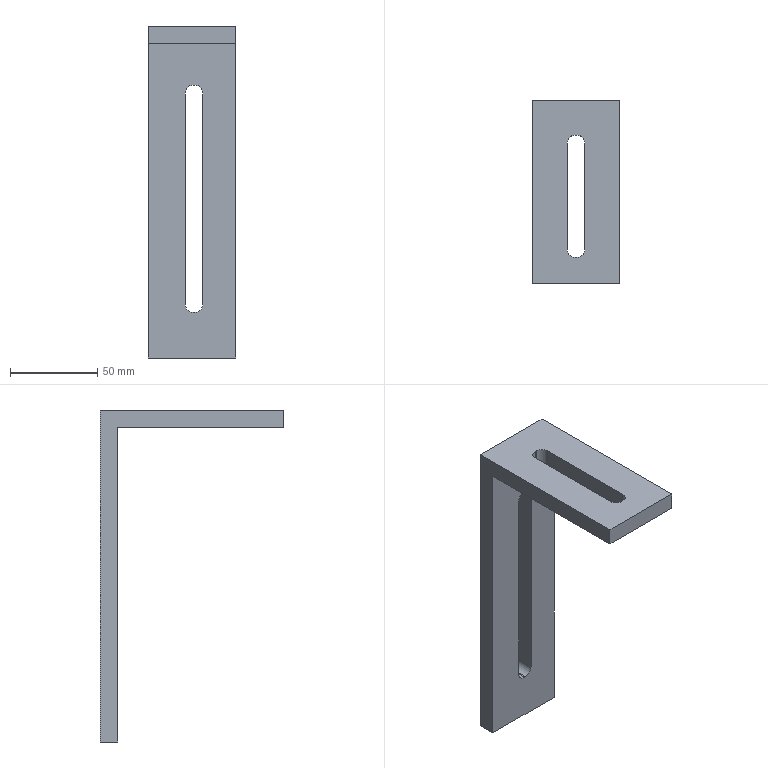Part | SolidWorks | features ICE 3, Extrusion 1 | 1 solid | 24 faces | box 50 x 105 x 190 mm | volume 122848 mm3 | plane 16 | cylinder 8 | commonest cylinder face diameters 9 x8
STEP:
#1=CARTESIAN_POINT('',(-25.,-50.,10.));
#2=VERTEX_POINT('',#1);
#3=CARTESIAN_POINT('',(-25.,-50.,0.));
#4=VERTEX_POINT('',#3);
#5=CARTESIAN_POINT('',(-25.,-50.,10.));
#6=DIRECTION('',(0.,0.,-1.));
#7=VECTOR('',#6,1000.);
#8=LINE('',#5,#7);
#9=EDGE_CURVE('',#2,#4,#8,.T.);
#10=ORIENTED_EDGE('',*,*,#9,.F.);
#11=CARTESIAN_POINT('',(-25.,55.,10.));
#12=VERTEX_POINT('',#11);
#13=CARTESIAN_POINT('',(-25.,-50.,10.));
#14=DIRECTION('',(0.,-1.,0.));
#15=VECTOR('',#14,1000.);
#16=LINE('',#13,#15);
#17=EDGE_CURVE('',#12,#2,#16,.T.);
#18=ORIENTED_EDGE('',*,*,#17,.F.);
#19=CARTESIAN_POINT('',(-25.,55.,-180.));
#20=VERTEX_POINT('',#19);
#21=CARTESIAN_POINT('',(-25.,55.,10.));
#22=DIRECTION('',(0.,0.,-1.));
#23=VECTOR('',#22,1000.);
#24=LINE('',#21,#23);
#25=EDGE_CURVE('',#12,#20,#24,.T.);
#26=ORIENTED_EDGE('',*,*,#25,.T.);
#27=CARTESIAN_POINT('',(-25.,45.,-180.));
#28=VERTEX_POINT('',#27);
#29=CARTESIAN_POINT('',(-25.,45.,-180.));
#30=DIRECTION('',(0.,1.,0.));
#31=VECTOR('',#30,1000.);
#32=LINE('',#29,#31);
#33=EDGE_CURVE('',#28,#20,#32,.T.);
#34=ORIENTED_EDGE('',*,*,#33,.F.);
#35=CARTESIAN_POINT('',(-25.,45.,0.));
#36=VERTEX_POINT('',#35);
#37=CARTESIAN_POINT('',(-25.,45.,10.));
#38=DIRECTION('',(0.,0.,-1.));
#39=VECTOR('',#38,1000.);
#40=LINE('',#37,#39);
#41=EDGE_CURVE('',#36,#28,#40,.T.);
#42=ORIENTED_EDGE('',*,*,#41,.F.);
#43=CARTESIAN_POINT('',(-25.,-50.,0.));
#44=DIRECTION('',(0.,-1.,0.));
#45=VECTOR('',#44,1000.);
#46=LINE('',#43,#45);
#47=EDGE_CURVE('',#36,#4,#46,.T.);
#48=ORIENTED_EDGE('',*,*,#47,.T.);
#49=EDGE_LOOP('',(#10,#18,#26,#34,#42,#48));
#50=FACE_OUTER_BOUND('',#49,.T.);
#51=CARTESIAN_POINT('',(-25.,-50.,10.));
#52=DIRECTION('',(1.,0.,0.));
#53=DIRECTION('',(0.,0.,-1.));
#54=AXIS2_PLACEMENT_3D('',#51,#52,#53);
#55=PLANE('',#54);
#56=ADVANCED_FACE('',(#50),#55,.F.);
#57=CARTESIAN_POINT('',(25.,-50.,0.));
#58=VERTEX_POINT('',#57);
#59=CARTESIAN_POINT('',(25.,-50.,0.));
#60=DIRECTION('',(1.,0.,0.));
#61=VECTOR('',#60,1000.);
#62=LINE('',#59,#61);
#63=EDGE_CURVE('',#4,#58,#62,.T.);
#64=ORIENTED_EDGE('',*,*,#63,.T.);
#65=CARTESIAN_POINT('',(25.,-50.,10.));
#66=VERTEX_POINT('',#65);
#67=CARTESIAN_POINT('',(25.,-50.,10.));
#68=DIRECTION('',(0.,0.,-1.));
#69=VECTOR('',#68,1000.);
#70=LINE('',#67,#69);
#71=EDGE_CURVE('',#66,#58,#70,.T.);
#72=ORIENTED_EDGE('',*,*,#71,.F.);
#73=CARTESIAN_POINT('',(25.,-50.,10.));
#74=DIRECTION('',(1.,0.,0.));
#75=VECTOR('',#74,1000.);
#76=LINE('',#73,#75);
#77=EDGE_CURVE('',#2,#66,#76,.T.);
#78=ORIENTED_EDGE('',*,*,#77,.F.);
#79=ORIENTED_EDGE('',*,*,#9,.T.);
#80=EDGE_LOOP('',(#64,#72,#78,#79));
#81=FACE_OUTER_BOUND('',#80,.T.);
#82=CARTESIAN_POINT('',(25.,-50.,10.));
#83=DIRECTION('',(0.,1.,0.));
#84=DIRECTION('',(0.,0.,1.));
#85=AXIS2_PLACEMENT_3D('',#82,#83,#84);
#86=PLANE('',#85);
#87=ADVANCED_FACE('',(#81),#86,.F.);
#88=CARTESIAN_POINT('',(25.,45.,0.));
#89=VERTEX_POINT('',#88);
#90=CARTESIAN_POINT('',(25.,-50.,0.));
#91=DIRECTION('',(0.,1.,0.));
#92=VECTOR('',#91,1000.);
#93=LINE('',#90,#92);
#94=EDGE_CURVE('',#58,#89,#93,.T.);
#95=ORIENTED_EDGE('',*,*,#94,.T.);
#96=CARTESIAN_POINT('',(25.,45.,-180.));
#97=VERTEX_POINT('',#96);
#98=CARTESIAN_POINT('',(25.,45.,10.));
#99=DIRECTION('',(0.,0.,-1.));
#100=VECTOR('',#99,1000.);
#101=LINE('',#98,#100);
#102=EDGE_CURVE('',#89,#97,#101,.T.);
#103=ORIENTED_EDGE('',*,*,#102,.T.);
#104=CARTESIAN_POINT('',(25.,55.,-180.));
#105=VERTEX_POINT('',#104);
#106=CARTESIAN_POINT('',(25.,45.,-180.));
#107=DIRECTION('',(0.,-1.,0.));
#108=VECTOR('',#107,1000.);
#109=LINE('',#106,#108);
#110=EDGE_CURVE('',#105,#97,#109,.T.);
#111=ORIENTED_EDGE('',*,*,#110,.F.);
#112=CARTESIAN_POINT('',(25.,55.,10.));
#113=VERTEX_POINT('',#112);
#114=CARTESIAN_POINT('',(25.,55.,10.));
#115=DIRECTION('',(0.,0.,-1.));
#116=VECTOR('',#115,1000.);
#117=LINE('',#114,#116);
#118=EDGE_CURVE('',#113,#105,#117,.T.);
#119=ORIENTED_EDGE('',*,*,#118,.F.);
#120=CARTESIAN_POINT('',(25.,-50.,10.));
#121=DIRECTION('',(0.,1.,0.));
#122=VECTOR('',#121,1000.);
#123=LINE('',#120,#122);
#124=EDGE_CURVE('',#66,#113,#123,.T.);
#125=ORIENTED_EDGE('',*,*,#124,.F.);
#126=ORIENTED_EDGE('',*,*,#71,.T.);
#127=EDGE_LOOP('',(#95,#103,#111,#119,#125,#126));
#128=FACE_OUTER_BOUND('',#127,.T.);
#129=CARTESIAN_POINT('',(25.,-50.,10.));
#130=DIRECTION('',(-1.,0.,0.));
#131=DIRECTION('',(0.,0.,1.));
#132=AXIS2_PLACEMENT_3D('',#129,#130,#131);
#133=PLANE('',#132);
#134=ADVANCED_FACE('',(#128),#133,.F.);
#135=ORIENTED_EDGE('',*,*,#124,.T.);
#136=CARTESIAN_POINT('',(-25.,55.,10.));
#137=DIRECTION('',(1.,0.,0.));
#138=VECTOR('',#137,1000.);
#139=LINE('',#136,#138);
#140=EDGE_CURVE('',#12,#113,#139,.T.);
#141=ORIENTED_EDGE('',*,*,#140,.F.);
#142=ORIENTED_EDGE('',*,*,#17,.T.);
#143=ORIENTED_EDGE('',*,*,#77,.T.);
#144=EDGE_LOOP('',(#135,#141,#142,#143));
#145=FACE_OUTER_BOUND('',#144,.T.);
#146=CARTESIAN_POINT('',(-5.,-30.5,10.));
#147=VERTEX_POINT('',#146);
#148=CARTESIAN_POINT('',(-0.5,-35.,10.));
#149=VERTEX_POINT('',#148);
#150=CARTESIAN_POINT('',(-0.5,-30.5,10.));
#151=DIRECTION('',(0.,0.,1.));
#152=DIRECTION('',(-1.,0.,0.));
#153=AXIS2_PLACEMENT_3D('',#150,#151,#152);
#154=CIRCLE('',#153,4.5);
#155=EDGE_CURVE('',#147,#149,#154,.T.);
#156=ORIENTED_EDGE('',*,*,#155,.F.);
#157=CARTESIAN_POINT('',(-5.,30.5,10.));
#158=VERTEX_POINT('',#157);
#159=CARTESIAN_POINT('',(-5.,-30.5,10.));
#160=DIRECTION('',(0.,-1.,0.));
#161=VECTOR('',#160,1000.);
#162=LINE('',#159,#161);
#163=EDGE_CURVE('',#158,#147,#162,.T.);
#164=ORIENTED_EDGE('',*,*,#163,.F.);
#165=CARTESIAN_POINT('',(-0.5,35.,10.));
#166=VERTEX_POINT('',#165);
#167=CARTESIAN_POINT('',(-0.5,30.5,10.));
#168=DIRECTION('',(0.,0.,1.));
#169=DIRECTION('',(1.,0.,0.));
#170=AXIS2_PLACEMENT_3D('',#167,#168,#169);
#171=CIRCLE('',#170,4.5);
#172=EDGE_CURVE('',#166,#158,#171,.T.);
#173=ORIENTED_EDGE('',*,*,#172,.F.);
#174=CARTESIAN_POINT('',(0.5,35.,10.));
#175=VERTEX_POINT('',#174);
#176=CARTESIAN_POINT('',(0.5,35.,10.));
#177=DIRECTION('',(-1.,0.,0.));
#178=VECTOR('',#177,1000.);
#179=LINE('',#176,#178);
#180=EDGE_CURVE('',#175,#166,#179,.T.);
#181=ORIENTED_EDGE('',*,*,#180,.F.);
#182=CARTESIAN_POINT('',(5.,30.5,10.));
#183=VERTEX_POINT('',#182);
#184=CARTESIAN_POINT('',(0.5,30.5,10.));
#185=DIRECTION('',(0.,0.,1.));
#186=DIRECTION('',(1.,0.,0.));
#187=AXIS2_PLACEMENT_3D('',#184,#185,#186);
#188=CIRCLE('',#187,4.5);
#189=EDGE_CURVE('',#183,#175,#188,.T.);
#190=ORIENTED_EDGE('',*,*,#189,.F.);
#191=CARTESIAN_POINT('',(5.,-30.5,10.));
#192=VERTEX_POINT('',#191);
#193=CARTESIAN_POINT('',(5.,-30.5,10.));
#194=DIRECTION('',(0.,1.,0.));
#195=VECTOR('',#194,1000.);
#196=LINE('',#193,#195);
#197=EDGE_CURVE('',#192,#183,#196,.T.);
#198=ORIENTED_EDGE('',*,*,#197,.F.);
#199=CARTESIAN_POINT('',(0.5,-35.,10.));
#200=VERTEX_POINT('',#199);
#201=CARTESIAN_POINT('',(0.5,-30.5,10.));
#202=DIRECTION('',(0.,0.,1.));
#203=DIRECTION('',(1.,0.,0.));
#204=AXIS2_PLACEMENT_3D('',#201,#202,#203);
#205=CIRCLE('',#204,4.5);
#206=EDGE_CURVE('',#200,#192,#205,.T.);
#207=ORIENTED_EDGE('',*,*,#206,.F.);
#208=CARTESIAN_POINT('',(0.5,-35.,10.));
#209=DIRECTION('',(1.,0.,0.));
#210=VECTOR('',#209,1000.);
#211=LINE('',#208,#210);
#212=EDGE_CURVE('',#149,#200,#211,.T.);
#213=ORIENTED_EDGE('',*,*,#212,.F.);
#214=EDGE_LOOP('',(#156,#164,#173,#181,#190,#198,#207,#213));
#215=FACE_BOUND('',#214,.T.);
#216=CARTESIAN_POINT('',(-25.,50.,10.));
#217=DIRECTION('',(0.,0.,1.));
#218=DIRECTION('',(1.,0.,0.));
#219=AXIS2_PLACEMENT_3D('',#216,#217,#218);
#220=PLANE('',#219);
#221=ADVANCED_FACE('',(#145,#215),#220,.T.);
#222=CARTESIAN_POINT('',(-5.,30.5,0.));
#223=VERTEX_POINT('',#222);
#224=CARTESIAN_POINT('',(-5.,-30.5,0.));
#225=VERTEX_POINT('',#224);
#226=CARTESIAN_POINT('',(-5.,-30.5,0.));
#227=DIRECTION('',(0.,-1.,0.));
#228=VECTOR('',#227,1000.);
#229=LINE('',#226,#228);
#230=EDGE_CURVE('',#223,#225,#229,.T.);
#231=ORIENTED_EDGE('',*,*,#230,.T.);
#232=CARTESIAN_POINT('',(-0.5,-35.,0.));
#233=VERTEX_POINT('',#232);
#234=CARTESIAN_POINT('',(-0.5,-30.5,0.));
#235=DIRECTION('',(0.,0.,1.));
#236=DIRECTION('',(-1.,0.,0.));
#237=AXIS2_PLACEMENT_3D('',#234,#235,#236);
#238=CIRCLE('',#237,4.5);
#239=EDGE_CURVE('',#225,#233,#238,.T.);
#240=ORIENTED_EDGE('',*,*,#239,.T.);
#241=CARTESIAN_POINT('',(0.5,-35.,0.));
#242=VERTEX_POINT('',#241);
#243=CARTESIAN_POINT('',(0.5,-35.,0.));
#244=DIRECTION('',(1.,0.,0.));
#245=VECTOR('',#244,1000.);
#246=LINE('',#243,#245);
#247=EDGE_CURVE('',#233,#242,#246,.T.);
#248=ORIENTED_EDGE('',*,*,#247,.T.);
#249=CARTESIAN_POINT('',(5.,-30.5,0.));
#250=VERTEX_POINT('',#249);
#251=CARTESIAN_POINT('',(0.5,-30.5,0.));
#252=DIRECTION('',(0.,0.,1.));
#253=DIRECTION('',(1.,0.,0.));
#254=AXIS2_PLACEMENT_3D('',#251,#252,#253);
#255=CIRCLE('',#254,4.5);
#256=EDGE_CURVE('',#242,#250,#255,.T.);
#257=ORIENTED_EDGE('',*,*,#256,.T.);
#258=CARTESIAN_POINT('',(5.,30.5,0.));
#259=VERTEX_POINT('',#258);
#260=CARTESIAN_POINT('',(5.,-30.5,0.));
#261=DIRECTION('',(0.,1.,0.));
#262=VECTOR('',#261,1000.);
#263=LINE('',#260,#262);
#264=EDGE_CURVE('',#250,#259,#263,.T.);
#265=ORIENTED_EDGE('',*,*,#264,.T.);
#266=CARTESIAN_POINT('',(0.5,35.,0.));
#267=VERTEX_POINT('',#266);
#268=CARTESIAN_POINT('',(0.5,30.5,0.));
#269=DIRECTION('',(0.,0.,1.));
#270=DIRECTION('',(1.,0.,0.));
#271=AXIS2_PLACEMENT_3D('',#268,#269,#270);
#272=CIRCLE('',#271,4.5);
#273=EDGE_CURVE('',#259,#267,#272,.T.);
#274=ORIENTED_EDGE('',*,*,#273,.T.);
#275=CARTESIAN_POINT('',(-0.5,35.,0.));
#276=VERTEX_POINT('',#275);
#277=CARTESIAN_POINT('',(0.5,35.,0.));
#278=DIRECTION('',(-1.,0.,0.));
#279=VECTOR('',#278,1000.);
#280=LINE('',#277,#279);
#281=EDGE_CURVE('',#267,#276,#280,.T.);
#282=ORIENTED_EDGE('',*,*,#281,.T.);
#283=CARTESIAN_POINT('',(-0.5,30.5,0.));
#284=DIRECTION('',(0.,0.,1.));
#285=DIRECTION('',(1.,0.,0.));
#286=AXIS2_PLACEMENT_3D('',#283,#284,#285);
#287=CIRCLE('',#286,4.5);
#288=EDGE_CURVE('',#276,#223,#287,.T.);
#289=ORIENTED_EDGE('',*,*,#288,.T.);
#290=EDGE_LOOP('',(#231,#240,#248,#257,#265,#274,#282,#289));
#291=FACE_BOUND('',#290,.T.);
#292=ORIENTED_EDGE('',*,*,#47,.F.);
#293=CARTESIAN_POINT('',(-25.,45.,0.));
#294=DIRECTION('',(1.,0.,0.));
#295=VECTOR('',#294,1000.);
#296=LINE('',#293,#295);
#297=EDGE_CURVE('',#36,#89,#296,.T.);
#298=ORIENTED_EDGE('',*,*,#297,.T.);
#299=ORIENTED_EDGE('',*,*,#94,.F.);
#300=ORIENTED_EDGE('',*,*,#63,.F.);
#301=EDGE_LOOP('',(#292,#298,#299,#300));
#302=FACE_OUTER_BOUND('',#301,.T.);
#303=CARTESIAN_POINT('',(-25.,50.,0.));
#304=DIRECTION('',(0.,0.,1.));
#305=DIRECTION('',(1.,0.,0.));
#306=AXIS2_PLACEMENT_3D('',#303,#304,#305);
#307=PLANE('',#306);
#308=ADVANCED_FACE('',(#291,#302),#307,.F.);
#309=ORIENTED_EDGE('',*,*,#155,.T.);
#310=CARTESIAN_POINT('',(-0.5,-35.,0.));
#311=DIRECTION('',(0.,0.,1.));
#312=VECTOR('',#311,1000.);
#313=LINE('',#310,#312);
#314=EDGE_CURVE('',#233,#149,#313,.T.);
#315=ORIENTED_EDGE('',*,*,#314,.F.);
#316=ORIENTED_EDGE('',*,*,#239,.F.);
#317=CARTESIAN_POINT('',(-5.,-30.5,0.));
#318=DIRECTION('',(0.,0.,1.));
#319=VECTOR('',#318,1000.);
#320=LINE('',#317,#319);
#321=EDGE_CURVE('',#225,#147,#320,.T.);
#322=ORIENTED_EDGE('',*,*,#321,.T.);
#323=EDGE_LOOP('',(#309,#315,#316,#322));
#324=FACE_OUTER_BOUND('',#323,.T.);
#325=CARTESIAN_POINT('',(-0.5,-30.5,0.));
#326=DIRECTION('',(0.,0.,1.));
#327=DIRECTION('',(1.,0.,0.));
#328=AXIS2_PLACEMENT_3D('',#325,#326,#327);
#329=CYLINDRICAL_SURFACE('',#328,4.5);
#330=ADVANCED_FACE('',(#324),#329,.F.);
#331=ORIENTED_EDGE('',*,*,#163,.T.);
#332=ORIENTED_EDGE('',*,*,#321,.F.);
#333=ORIENTED_EDGE('',*,*,#230,.F.);
#334=CARTESIAN_POINT('',(-5.,30.5,0.));
#335=DIRECTION('',(0.,0.,1.));
#336=VECTOR('',#335,1000.);
#337=LINE('',#334,#336);
#338=EDGE_CURVE('',#223,#158,#337,.T.);
#339=ORIENTED_EDGE('',*,*,#338,.T.);
#340=EDGE_LOOP('',(#331,#332,#333,#339));
#341=FACE_OUTER_BOUND('',#340,.T.);
#342=CARTESIAN_POINT('',(-5.,-30.5,0.));
#343=DIRECTION('',(-1.,0.,0.));
#344=DIRECTION('',(0.,0.,1.));
#345=AXIS2_PLACEMENT_3D('',#342,#343,#344);
#346=PLANE('',#345);
#347=ADVANCED_FACE('',(#341),#346,.F.);
#348=ORIENTED_EDGE('',*,*,#172,.T.);
#349=ORIENTED_EDGE('',*,*,#338,.F.);
#350=ORIENTED_EDGE('',*,*,#288,.F.);
#351=CARTESIAN_POINT('',(-0.5,35.,0.));
#352=DIRECTION('',(0.,0.,1.));
#353=VECTOR('',#352,1000.);
#354=LINE('',#351,#353);
#355=EDGE_CURVE('',#276,#166,#354,.T.);
#356=ORIENTED_EDGE('',*,*,#355,.T.);
#357=EDGE_LOOP('',(#348,#349,#350,#356));
#358=FACE_OUTER_BOUND('',#357,.T.);
#359=CARTESIAN_POINT('',(-0.5,30.5,0.));
#360=DIRECTION('',(0.,0.,1.));
#361=DIRECTION('',(1.,0.,0.));
#362=AXIS2_PLACEMENT_3D('',#359,#360,#361);
#363=CYLINDRICAL_SURFACE('',#362,4.5);
#364=ADVANCED_FACE('',(#358),#363,.F.);
#365=ORIENTED_EDGE('',*,*,#180,.T.);
#366=ORIENTED_EDGE('',*,*,#355,.F.);
#367=ORIENTED_EDGE('',*,*,#281,.F.);
#368=CARTESIAN_POINT('',(0.5,35.,0.));
#369=DIRECTION('',(0.,0.,1.));
#370=VECTOR('',#369,1000.);
#371=LINE('',#368,#370);
#372=EDGE_CURVE('',#267,#175,#371,.T.);
#373=ORIENTED_EDGE('',*,*,#372,.T.);
#374=EDGE_LOOP('',(#365,#366,#367,#373));
#375=FACE_OUTER_BOUND('',#374,.T.);
#376=CARTESIAN_POINT('',(0.5,35.,0.));
#377=DIRECTION('',(0.,1.,0.));
#378=DIRECTION('',(0.,0.,1.));
#379=AXIS2_PLACEMENT_3D('',#376,#377,#378);
#380=PLANE('',#379);
#381=ADVANCED_FACE('',(#375),#380,.F.);
#382=ORIENTED_EDGE('',*,*,#189,.T.);
#383=ORIENTED_EDGE('',*,*,#372,.F.);
#384=ORIENTED_EDGE('',*,*,#273,.F.);
#385=CARTESIAN_POINT('',(5.,30.5,0.));
#386=DIRECTION('',(0.,0.,1.));
#387=VECTOR('',#386,1000.);
#388=LINE('',#385,#387);
#389=EDGE_CURVE('',#259,#183,#388,.T.);
#390=ORIENTED_EDGE('',*,*,#389,.T.);
#391=EDGE_LOOP('',(#382,#383,#384,#390));
#392=FACE_OUTER_BOUND('',#391,.T.);
#393=CARTESIAN_POINT('',(0.5,30.5,0.));
#394=DIRECTION('',(0.,0.,1.));
#395=DIRECTION('',(1.,0.,0.));
#396=AXIS2_PLACEMENT_3D('',#393,#394,#395);
#397=CYLINDRICAL_SURFACE('',#396,4.5);
#398=ADVANCED_FACE('',(#392),#397,.F.);
#399=ORIENTED_EDGE('',*,*,#197,.T.);
#400=ORIENTED_EDGE('',*,*,#389,.F.);
#401=ORIENTED_EDGE('',*,*,#264,.F.);
#402=CARTESIAN_POINT('',(5.,-30.5,0.));
#403=DIRECTION('',(0.,0.,1.));
#404=VECTOR('',#403,1000.);
#405=LINE('',#402,#404);
#406=EDGE_CURVE('',#250,#192,#405,.T.);
#407=ORIENTED_EDGE('',*,*,#406,.T.);
#408=EDGE_LOOP('',(#399,#400,#401,#407));
#409=FACE_OUTER_BOUND('',#408,.T.);
#410=CARTESIAN_POINT('',(5.,-30.5,0.));
#411=DIRECTION('',(1.,0.,0.));
#412=DIRECTION('',(0.,0.,-1.));
#413=AXIS2_PLACEMENT_3D('',#410,#411,#412);
#414=PLANE('',#413);
#415=ADVANCED_FACE('',(#409),#414,.F.);
#416=ORIENTED_EDGE('',*,*,#206,.T.);
#417=ORIENTED_EDGE('',*,*,#406,.F.);
#418=ORIENTED_EDGE('',*,*,#256,.F.);
#419=CARTESIAN_POINT('',(0.5,-35.,0.));
#420=DIRECTION('',(0.,0.,1.));
#421=VECTOR('',#420,1000.);
#422=LINE('',#419,#421);
#423=EDGE_CURVE('',#242,#200,#422,.T.);
#424=ORIENTED_EDGE('',*,*,#423,.T.);
#425=EDGE_LOOP('',(#416,#417,#418,#424));
#426=FACE_OUTER_BOUND('',#425,.T.);
#427=CARTESIAN_POINT('',(0.5,-30.5,0.));
#428=DIRECTION('',(0.,0.,1.));
#429=DIRECTION('',(1.,0.,0.));
#430=AXIS2_PLACEMENT_3D('',#427,#428,#429);
#431=CYLINDRICAL_SURFACE('',#430,4.5);
#432=ADVANCED_FACE('',(#426),#431,.F.);
#433=ORIENTED_EDGE('',*,*,#212,.T.);
#434=ORIENTED_EDGE('',*,*,#423,.F.);
#435=ORIENTED_EDGE('',*,*,#247,.F.);
#436=ORIENTED_EDGE('',*,*,#314,.T.);
#437=EDGE_LOOP('',(#433,#434,#435,#436));
#438=FACE_OUTER_BOUND('',#437,.T.);
#439=CARTESIAN_POINT('',(0.5,-35.,0.));
#440=DIRECTION('',(0.,-1.,0.));
#441=DIRECTION('',(0.,0.,-1.));
#442=AXIS2_PLACEMENT_3D('',#439,#440,#441);
#443=PLANE('',#442);
#444=ADVANCED_FACE('',(#438),#443,.F.);
#445=CARTESIAN_POINT('',(1.635,45.,-153.843));
#446=VERTEX_POINT('',#445);
#447=CARTESIAN_POINT('',(6.135,45.,-149.343));
#448=VERTEX_POINT('',#447);
#449=CARTESIAN_POINT('',(1.635,45.,-149.343));
#450=DIRECTION('',(0.,-1.,0.));
#451=DIRECTION('',(0.,0.,-1.));
#452=AXIS2_PLACEMENT_3D('',#449,#450,#451);
#453=CIRCLE('',#452,4.5);
#454=EDGE_CURVE('',#446,#448,#453,.T.);
#455=ORIENTED_EDGE('',*,*,#454,.F.);
#456=CARTESIAN_POINT('',(0.6349,45.,-153.843));
#457=VERTEX_POINT('',#456);
#458=CARTESIAN_POINT('',(1.635,45.,-153.843));
#459=DIRECTION('',(1.,0.,0.));
#460=VECTOR('',#459,1000.);
#461=LINE('',#458,#460);
#462=EDGE_CURVE('',#457,#446,#461,.T.);
#463=ORIENTED_EDGE('',*,*,#462,.F.);
#464=CARTESIAN_POINT('',(-3.865,45.,-149.343));
#465=VERTEX_POINT('',#464);
#466=CARTESIAN_POINT('',(0.6349,45.,-149.343));
#467=DIRECTION('',(0.,-1.,0.));
#468=DIRECTION('',(0.,0.,1.));
#469=AXIS2_PLACEMENT_3D('',#466,#467,#468);
#470=CIRCLE('',#469,4.5);
#471=EDGE_CURVE('',#465,#457,#470,.T.);
#472=ORIENTED_EDGE('',*,*,#471,.F.);
#473=CARTESIAN_POINT('',(-3.865,45.,-28.343));
#474=VERTEX_POINT('',#473);
#475=CARTESIAN_POINT('',(-3.865,45.,-149.343));
#476=DIRECTION('',(0.,0.,-1.));
#477=VECTOR('',#476,1000.);
#478=LINE('',#475,#477);
#479=EDGE_CURVE('',#474,#465,#478,.T.);
#480=ORIENTED_EDGE('',*,*,#479,.F.);
#481=CARTESIAN_POINT('',(0.6349,45.,-23.843));
#482=VERTEX_POINT('',#481);
#483=CARTESIAN_POINT('',(0.6349,45.,-28.343));
#484=DIRECTION('',(0.,-1.,0.));
#485=DIRECTION('',(0.,0.,-1.));
#486=AXIS2_PLACEMENT_3D('',#483,#484,#485);
#487=CIRCLE('',#486,4.5);
#488=EDGE_CURVE('',#482,#474,#487,.T.);
#489=ORIENTED_EDGE('',*,*,#488,.F.);
#490=CARTESIAN_POINT('',(1.635,45.,-23.843));
#491=VERTEX_POINT('',#490);
#492=CARTESIAN_POINT('',(1.635,45.,-23.843));
#493=DIRECTION('',(-1.,0.,0.));
#494=VECTOR('',#493,1000.);
#495=LINE('',#492,#494);
#496=EDGE_CURVE('',#491,#482,#495,.T.);
#497=ORIENTED_EDGE('',*,*,#496,.F.);
#498=CARTESIAN_POINT('',(6.135,45.,-28.343));
#499=VERTEX_POINT('',#498);
#500=CARTESIAN_POINT('',(1.635,45.,-28.343));
#501=DIRECTION('',(0.,-1.,0.));
#502=DIRECTION('',(0.,0.,-1.));
#503=AXIS2_PLACEMENT_3D('',#500,#501,#502);
#504=CIRCLE('',#503,4.5);
#505=EDGE_CURVE('',#499,#491,#504,.T.);
#506=ORIENTED_EDGE('',*,*,#505,.F.);
#507=CARTESIAN_POINT('',(6.135,45.,-149.343));
#508=DIRECTION('',(0.,0.,1.));
#509=VECTOR('',#508,1000.);
#510=LINE('',#507,#509);
#511=EDGE_CURVE('',#448,#499,#510,.T.);
#512=ORIENTED_EDGE('',*,*,#511,.F.);
#513=EDGE_LOOP('',(#455,#463,#472,#480,#489,#497,#506,#512));
#514=FACE_BOUND('',#513,.T.);
#515=ORIENTED_EDGE('',*,*,#297,.F.);
#516=ORIENTED_EDGE('',*,*,#41,.T.);
#517=CARTESIAN_POINT('',(-25.,45.,-180.));
#518=DIRECTION('',(-1.,0.,0.));
#519=VECTOR('',#518,1000.);
#520=LINE('',#517,#519);
#521=EDGE_CURVE('',#97,#28,#520,.T.);
#522=ORIENTED_EDGE('',*,*,#521,.F.);
#523=ORIENTED_EDGE('',*,*,#102,.F.);
#524=EDGE_LOOP('',(#515,#516,#522,#523));
#525=FACE_OUTER_BOUND('',#524,.T.);
#526=CARTESIAN_POINT('',(-25.,45.,10.));
#527=DIRECTION('',(0.,-1.,0.));
#528=DIRECTION('',(0.,0.,-1.));
#529=AXIS2_PLACEMENT_3D('',#526,#527,#528);
#530=PLANE('',#529);
#531=ADVANCED_FACE('',(#514,#525),#530,.T.);
#532=CARTESIAN_POINT('',(6.135,55.,-149.343));
#533=VERTEX_POINT('',#532);
#534=CARTESIAN_POINT('',(1.635,55.,-153.843));
#535=VERTEX_POINT('',#534);
#536=CARTESIAN_POINT('',(1.635,55.,-149.343));
#537=DIRECTION('',(0.,1.,0.));
#538=DIRECTION('',(0.,0.,1.));
#539=AXIS2_PLACEMENT_3D('',#536,#537,#538);
#540=CIRCLE('',#539,4.5);
#541=EDGE_CURVE('',#533,#535,#540,.T.);
#542=ORIENTED_EDGE('',*,*,#541,.F.);
#543=CARTESIAN_POINT('',(6.135,55.,-28.343));
#544=VERTEX_POINT('',#543);
#545=CARTESIAN_POINT('',(6.135,55.,10.));
#546=DIRECTION('',(0.,0.,-1.));
#547=VECTOR('',#546,1000.);
#548=LINE('',#545,#547);
#549=EDGE_CURVE('',#544,#533,#548,.T.);
#550=ORIENTED_EDGE('',*,*,#549,.F.);
#551=CARTESIAN_POINT('',(1.635,55.,-23.843));
#552=VERTEX_POINT('',#551);
#553=CARTESIAN_POINT('',(1.635,55.,-28.343));
#554=DIRECTION('',(0.,1.,0.));
#555=DIRECTION('',(0.,0.,1.));
#556=AXIS2_PLACEMENT_3D('',#553,#554,#555);
#557=CIRCLE('',#556,4.5);
#558=EDGE_CURVE('',#552,#544,#557,.T.);
#559=ORIENTED_EDGE('',*,*,#558,.F.);
#560=CARTESIAN_POINT('',(0.6349,55.,-23.843));
#561=VERTEX_POINT('',#560);
#562=CARTESIAN_POINT('',(-25.,55.,-23.843));
#563=DIRECTION('',(1.,0.,0.));
#564=VECTOR('',#563,1000.);
#565=LINE('',#562,#564);
#566=EDGE_CURVE('',#561,#552,#565,.T.);
#567=ORIENTED_EDGE('',*,*,#566,.F.);
#568=CARTESIAN_POINT('',(-3.865,55.,-28.343));
#569=VERTEX_POINT('',#568);
#570=CARTESIAN_POINT('',(0.6349,55.,-28.343));
#571=DIRECTION('',(0.,1.,0.));
#572=DIRECTION('',(0.,0.,1.));
#573=AXIS2_PLACEMENT_3D('',#570,#571,#572);
#574=CIRCLE('',#573,4.5);
#575=EDGE_CURVE('',#569,#561,#574,.T.);
#576=ORIENTED_EDGE('',*,*,#575,.F.);
#577=CARTESIAN_POINT('',(-3.865,55.,-149.343));
#578=VERTEX_POINT('',#577);
#579=CARTESIAN_POINT('',(-3.865,55.,10.));
#580=DIRECTION('',(0.,0.,1.));
#581=VECTOR('',#580,1000.);
#582=LINE('',#579,#581);
#583=EDGE_CURVE('',#578,#569,#582,.T.);
#584=ORIENTED_EDGE('',*,*,#583,.F.);
#585=CARTESIAN_POINT('',(0.6349,55.,-153.843));
#586=VERTEX_POINT('',#585);
#587=CARTESIAN_POINT('',(0.6349,55.,-149.343));
#588=DIRECTION('',(0.,1.,0.));
#589=DIRECTION('',(0.,0.,1.));
#590=AXIS2_PLACEMENT_3D('',#587,#588,#589);
#591=CIRCLE('',#590,4.5);
#592=EDGE_CURVE('',#586,#578,#591,.T.);
#593=ORIENTED_EDGE('',*,*,#592,.F.);
#594=CARTESIAN_POINT('',(-25.,55.,-153.843));
#595=DIRECTION('',(-1.,0.,0.));
#596=VECTOR('',#595,1000.);
#597=LINE('',#594,#596);
#598=EDGE_CURVE('',#535,#586,#597,.T.);
#599=ORIENTED_EDGE('',*,*,#598,.F.);
#600=EDGE_LOOP('',(#542,#550,#559,#567,#576,#584,#593,#599));
#601=FACE_BOUND('',#600,.T.);
#602=ORIENTED_EDGE('',*,*,#118,.T.);
#603=CARTESIAN_POINT('',(-25.,55.,-180.));
#604=DIRECTION('',(1.,0.,0.));
#605=VECTOR('',#604,1000.);
#606=LINE('',#603,#605);
#607=EDGE_CURVE('',#20,#105,#606,.T.);
#608=ORIENTED_EDGE('',*,*,#607,.F.);
#609=ORIENTED_EDGE('',*,*,#25,.F.);
#610=ORIENTED_EDGE('',*,*,#140,.T.);
#611=EDGE_LOOP('',(#602,#608,#609,#610));
#612=FACE_OUTER_BOUND('',#611,.T.);
#613=CARTESIAN_POINT('',(-25.,55.,10.));
#614=DIRECTION('',(0.,1.,0.));
#615=DIRECTION('',(0.,0.,1.));
#616=AXIS2_PLACEMENT_3D('',#613,#614,#615);
#617=PLANE('',#616);
#618=ADVANCED_FACE('',(#601,#612),#617,.T.);
#619=ORIENTED_EDGE('',*,*,#110,.T.);
#620=ORIENTED_EDGE('',*,*,#521,.T.);
#621=ORIENTED_EDGE('',*,*,#33,.T.);
#622=ORIENTED_EDGE('',*,*,#607,.T.);
#623=EDGE_LOOP('',(#619,#620,#621,#622));
#624=FACE_OUTER_BOUND('',#623,.T.);
#625=CARTESIAN_POINT('',(25.,55.,-180.));
#626=DIRECTION('',(0.,0.,-1.));
#627=DIRECTION('',(-1.,0.,0.));
#628=AXIS2_PLACEMENT_3D('',#625,#626,#627);
#629=PLANE('',#628);
#630=ADVANCED_FACE('',(#624),#629,.T.);
#631=ORIENTED_EDGE('',*,*,#541,.T.);
#632=CARTESIAN_POINT('',(1.635,225.,-153.843));
#633=DIRECTION('',(0.,-1.,0.));
#634=VECTOR('',#633,1000.);
#635=LINE('',#632,#634);
#636=EDGE_CURVE('',#535,#446,#635,.T.);
#637=ORIENTED_EDGE('',*,*,#636,.T.);
#638=ORIENTED_EDGE('',*,*,#454,.T.);
#639=CARTESIAN_POINT('',(6.135,225.,-149.343));
#640=DIRECTION('',(0.,-1.,0.));
#641=VECTOR('',#640,1000.);
#642=LINE('',#639,#641);
#643=EDGE_CURVE('',#533,#448,#642,.T.);
#644=ORIENTED_EDGE('',*,*,#643,.F.);
#645=EDGE_LOOP('',(#631,#637,#638,#644));
#646=FACE_OUTER_BOUND('',#645,.T.);
#647=CARTESIAN_POINT('',(1.635,225.,-149.343));
#648=DIRECTION('',(0.,-1.,0.));
#649=DIRECTION('',(0.,0.,-1.));
#650=AXIS2_PLACEMENT_3D('',#647,#648,#649);
#651=CYLINDRICAL_SURFACE('',#650,4.5);
#652=ADVANCED_FACE('',(#646),#651,.F.);
#653=ORIENTED_EDGE('',*,*,#598,.T.);
#654=CARTESIAN_POINT('',(0.6349,225.,-153.843));
#655=DIRECTION('',(0.,-1.,0.));
#656=VECTOR('',#655,1000.);
#657=LINE('',#654,#656);
#658=EDGE_CURVE('',#586,#457,#657,.T.);
#659=ORIENTED_EDGE('',*,*,#658,.T.);
#660=ORIENTED_EDGE('',*,*,#462,.T.);
#661=ORIENTED_EDGE('',*,*,#636,.F.);
#662=EDGE_LOOP('',(#653,#659,#660,#661));
#663=FACE_OUTER_BOUND('',#662,.T.);
#664=CARTESIAN_POINT('',(1.635,225.,-153.843));
#665=DIRECTION('',(0.,0.,-1.));
#666=DIRECTION('',(-1.,0.,0.));
#667=AXIS2_PLACEMENT_3D('',#664,#665,#666);
#668=PLANE('',#667);
#669=ADVANCED_FACE('',(#663),#668,.F.);
#670=ORIENTED_EDGE('',*,*,#592,.T.);
#671=CARTESIAN_POINT('',(-3.865,225.,-149.343));
#672=DIRECTION('',(0.,-1.,0.));
#673=VECTOR('',#672,1000.);
#674=LINE('',#671,#673);
#675=EDGE_CURVE('',#578,#465,#674,.T.);
#676=ORIENTED_EDGE('',*,*,#675,.T.);
#677=ORIENTED_EDGE('',*,*,#471,.T.);
#678=ORIENTED_EDGE('',*,*,#658,.F.);
#679=EDGE_LOOP('',(#670,#676,#677,#678));
#680=FACE_OUTER_BOUND('',#679,.T.);
#681=CARTESIAN_POINT('',(0.6349,225.,-149.343));
#682=DIRECTION('',(0.,-1.,0.));
#683=DIRECTION('',(0.,0.,-1.));
#684=AXIS2_PLACEMENT_3D('',#681,#682,#683);
#685=CYLINDRICAL_SURFACE('',#684,4.5);
#686=ADVANCED_FACE('',(#680),#685,.F.);
#687=ORIENTED_EDGE('',*,*,#583,.T.);
#688=CARTESIAN_POINT('',(-3.865,225.,-28.343));
#689=DIRECTION('',(0.,-1.,0.));
#690=VECTOR('',#689,1000.);
#691=LINE('',#688,#690);
#692=EDGE_CURVE('',#569,#474,#691,.T.);
#693=ORIENTED_EDGE('',*,*,#692,.T.);
#694=ORIENTED_EDGE('',*,*,#479,.T.);
#695=ORIENTED_EDGE('',*,*,#675,.F.);
#696=EDGE_LOOP('',(#687,#693,#694,#695));
#697=FACE_OUTER_BOUND('',#696,.T.);
#698=CARTESIAN_POINT('',(-3.865,225.,-149.343));
#699=DIRECTION('',(-1.,0.,0.));
#700=DIRECTION('',(0.,0.,1.));
#701=AXIS2_PLACEMENT_3D('',#698,#699,#700);
#702=PLANE('',#701);
#703=ADVANCED_FACE('',(#697),#702,.F.);
#704=ORIENTED_EDGE('',*,*,#575,.T.);
#705=CARTESIAN_POINT('',(0.6349,225.,-23.843));
#706=DIRECTION('',(0.,-1.,0.));
#707=VECTOR('',#706,1000.);
#708=LINE('',#705,#707);
#709=EDGE_CURVE('',#561,#482,#708,.T.);
#710=ORIENTED_EDGE('',*,*,#709,.T.);
#711=ORIENTED_EDGE('',*,*,#488,.T.);
#712=ORIENTED_EDGE('',*,*,#692,.F.);
#713=EDGE_LOOP('',(#704,#710,#711,#712));
#714=FACE_OUTER_BOUND('',#713,.T.);
#715=CARTESIAN_POINT('',(0.6349,225.,-28.343));
#716=DIRECTION('',(0.,-1.,0.));
#717=DIRECTION('',(0.,0.,-1.));
#718=AXIS2_PLACEMENT_3D('',#715,#716,#717);
#719=CYLINDRICAL_SURFACE('',#718,4.5);
#720=ADVANCED_FACE('',(#714),#719,.F.);
#721=ORIENTED_EDGE('',*,*,#566,.T.);
#722=CARTESIAN_POINT('',(1.635,225.,-23.843));
#723=DIRECTION('',(0.,-1.,0.));
#724=VECTOR('',#723,1000.);
#725=LINE('',#722,#724);
#726=EDGE_CURVE('',#552,#491,#725,.T.);
#727=ORIENTED_EDGE('',*,*,#726,.T.);
#728=ORIENTED_EDGE('',*,*,#496,.T.);
#729=ORIENTED_EDGE('',*,*,#709,.F.);
#730=EDGE_LOOP('',(#721,#727,#728,#729));
#731=FACE_OUTER_BOUND('',#730,.T.);
#732=CARTESIAN_POINT('',(1.635,225.,-23.843));
#733=DIRECTION('',(0.,0.,1.));
#734=DIRECTION('',(1.,0.,0.));
#735=AXIS2_PLACEMENT_3D('',#732,#733,#734);
#736=PLANE('',#735);
#737=ADVANCED_FACE('',(#731),#736,.F.);
#738=ORIENTED_EDGE('',*,*,#558,.T.);
#739=CARTESIAN_POINT('',(6.135,225.,-28.343));
#740=DIRECTION('',(0.,-1.,0.));
#741=VECTOR('',#740,1000.);
#742=LINE('',#739,#741);
#743=EDGE_CURVE('',#544,#499,#742,.T.);
#744=ORIENTED_EDGE('',*,*,#743,.T.);
#745=ORIENTED_EDGE('',*,*,#505,.T.);
#746=ORIENTED_EDGE('',*,*,#726,.F.);
#747=EDGE_LOOP('',(#738,#744,#745,#746));
#748=FACE_OUTER_BOUND('',#747,.T.);
#749=CARTESIAN_POINT('',(1.635,225.,-28.343));
#750=DIRECTION('',(0.,-1.,0.));
#751=DIRECTION('',(0.,0.,-1.));
#752=AXIS2_PLACEMENT_3D('',#749,#750,#751);
#753=CYLINDRICAL_SURFACE('',#752,4.5);
#754=ADVANCED_FACE('',(#748),#753,.F.);
#755=ORIENTED_EDGE('',*,*,#549,.T.);
#756=ORIENTED_EDGE('',*,*,#643,.T.);
#757=ORIENTED_EDGE('',*,*,#511,.T.);
#758=ORIENTED_EDGE('',*,*,#743,.F.);
#759=EDGE_LOOP('',(#755,#756,#757,#758));
#760=FACE_OUTER_BOUND('',#759,.T.);
#761=CARTESIAN_POINT('',(6.135,225.,-149.343));
#762=DIRECTION('',(1.,0.,0.));
#763=DIRECTION('',(0.,0.,-1.));
#764=AXIS2_PLACEMENT_3D('',#761,#762,#763);
#765=PLANE('',#764);
#766=ADVANCED_FACE('',(#760),#765,.F.);
#767=CLOSED_SHELL('',(#56,#87,#134,#221,#308,#330,#347,#364,#381,#398,#415,#432,#444,#531,#618,#630,#652,#669,#686,#703,#720,#737,#754,#766));
#768=MANIFOLD_SOLID_BREP('',#767);
#769=CARTESIAN_POINT('',(0.,0.,0.));
#770=DIRECTION('',(0.,0.,1.));
#771=DIRECTION('',(1.,0.,0.));
#772=AXIS2_PLACEMENT_3D('',#769,#770,#771);
#773=(LENGTH_UNIT()NAMED_UNIT(*)SI_UNIT(.MILLI.,.METRE.));
#774=UNCERTAINTY_MEASURE_WITH_UNIT(LENGTH_MEASURE(0.00001),#773,'','');
#775=(NAMED_UNIT(*)PLANE_ANGLE_UNIT()SI_UNIT($,.RADIAN.));
#776=(NAMED_UNIT(*)SI_UNIT($,.STERADIAN.)SOLID_ANGLE_UNIT());
#777=(GEOMETRIC_REPRESENTATION_CONTEXT(3)GLOBAL_UNCERTAINTY_ASSIGNED_CONTEXT((#774))GLOBAL_UNIT_ASSIGNED_CONTEXT((#773,#775,#776))REPRESENTATION_CONTEXT('',''));
#778=ADVANCED_BREP_SHAPE_REPRESENTATION('',(#768,#772),#777);